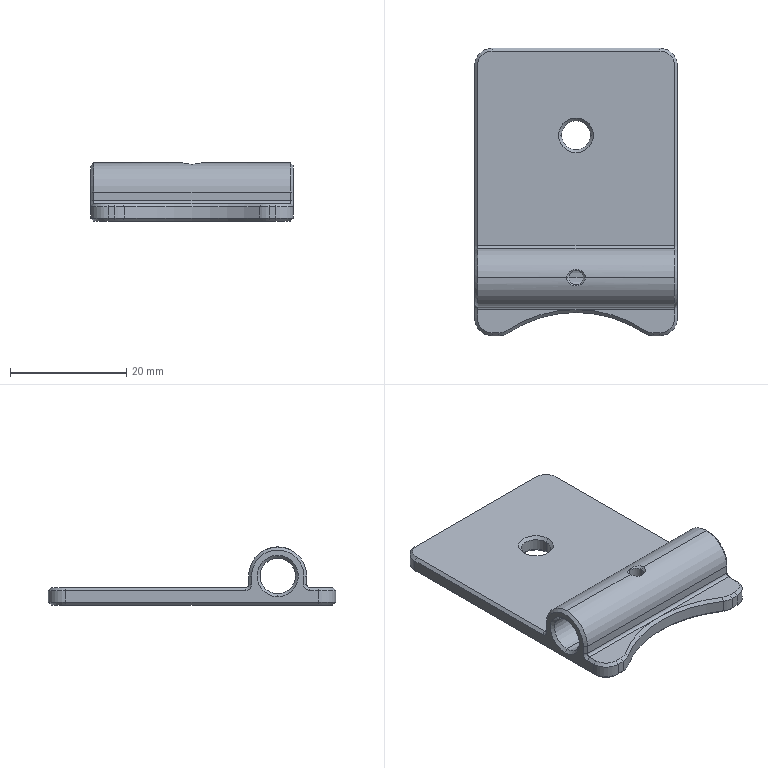Part | SolidWorks | features MoveFace 4, Fillet 2, 3DProfileFeature 1, Chamfer 1, DelFace 1, Extrusion 1, HoleWzd 1, ICE 1 | 1 solid | 75 faces | box 34.9 x 49.5 x 10 mm | volume 5888 mm3 | cone 31 | plane 27 | cylinder 17 | commonest cylinder face diameters 6 x6 1 x2 2.5 x2 5 x2 6.1 x2 10 x2